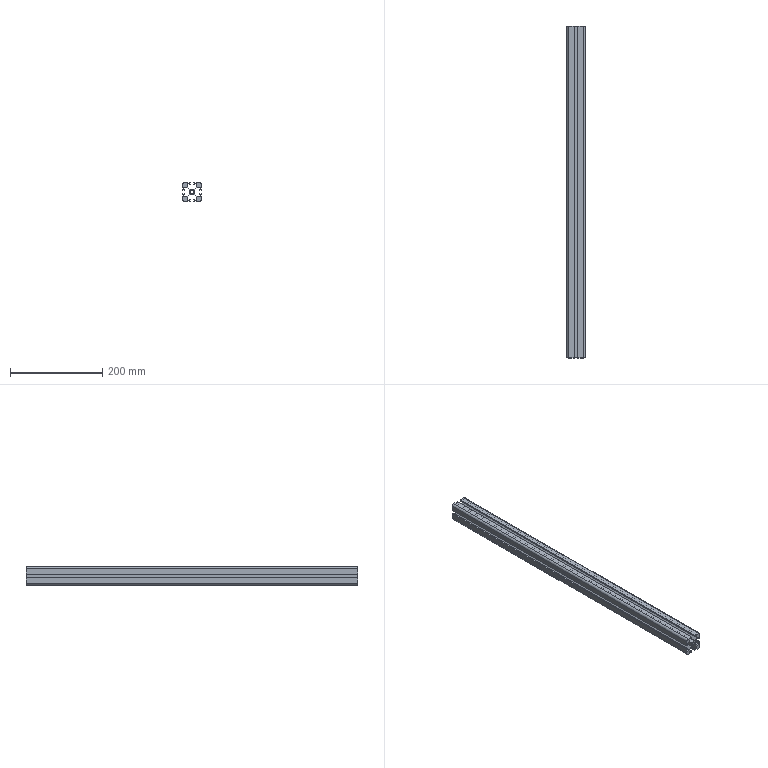Part | STEP file | 40x40-720 | 1 solid | 67 faces | box 40 x 720 x 40 mm | volume 397719 mm3 | plane 62 | cylinder 5 | commonest cylinder face diameters 9 x4 6.8 x1